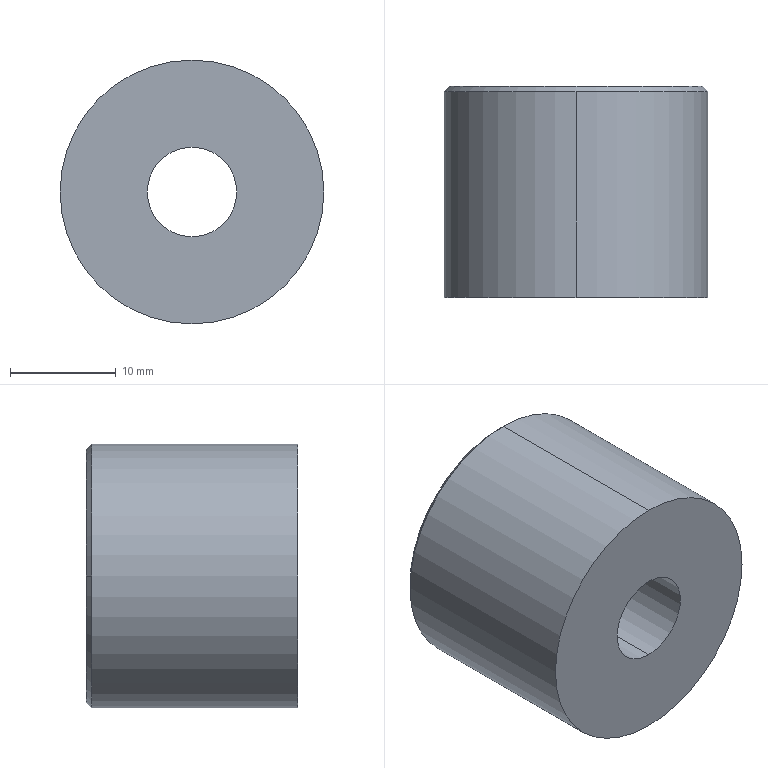Part | STEP file | VD-J260_10_1_1A_1-20_VD-SYL0380 | 1 solid | 8 faces | box 25 x 20 x 25 mm | volume 8673 mm3 | cylinder 4 | plane 2 | cone 2 | commonest cylinder face diameters 8.5 x2 25 x2
STEP:
#1=CARTESIAN_POINT('',(0.,0.,4.25));
#2=VERTEX_POINT('',#1);
#3=CARTESIAN_POINT('',(0.,0.,-4.25));
#4=VERTEX_POINT('',#3);
#5=CARTESIAN_POINT('',(0.,0.,0.));
#6=DIRECTION('',(0.,1.,0.));
#7=DIRECTION('',(0.,0.,1.));
#8=AXIS2_PLACEMENT_3D('',#5,#6,#7);
#9=CIRCLE('',#8,4.25);
#10=EDGE_CURVE('',#2,#4,#9,.T.);
#11=ORIENTED_EDGE('',*,*,#10,.F.);
#12=CARTESIAN_POINT('',(0.,20.,4.25));
#13=VERTEX_POINT('',#12);
#14=CARTESIAN_POINT('',(0.,20.,4.25));
#15=DIRECTION('',(0.,-1.,0.));
#16=VECTOR('',#15,1000.);
#17=LINE('',#14,#16);
#18=EDGE_CURVE('',#13,#2,#17,.T.);
#19=ORIENTED_EDGE('',*,*,#18,.F.);
#20=CARTESIAN_POINT('',(0.,20.,-4.25));
#21=VERTEX_POINT('',#20);
#22=CARTESIAN_POINT('',(0.,20.,0.));
#23=DIRECTION('',(0.,-1.,0.));
#24=DIRECTION('',(0.,0.,-1.));
#25=AXIS2_PLACEMENT_3D('',#22,#23,#24);
#26=CIRCLE('',#25,4.25);
#27=EDGE_CURVE('',#21,#13,#26,.T.);
#28=ORIENTED_EDGE('',*,*,#27,.F.);
#29=CARTESIAN_POINT('',(0.,20.,-4.25));
#30=DIRECTION('',(0.,-1.,0.));
#31=VECTOR('',#30,1000.);
#32=LINE('',#29,#31);
#33=EDGE_CURVE('',#21,#4,#32,.T.);
#34=ORIENTED_EDGE('',*,*,#33,.T.);
#35=EDGE_LOOP('',(#11,#19,#28,#34));
#36=FACE_OUTER_BOUND('',#35,.T.);
#37=CARTESIAN_POINT('',(0.,-14.181,0.));
#38=DIRECTION('',(0.,1.,0.));
#39=DIRECTION('',(0.,0.,1.));
#40=AXIS2_PLACEMENT_3D('',#37,#38,#39);
#41=CYLINDRICAL_SURFACE('',#40,4.25);
#42=ADVANCED_FACE('',(#36),#41,.F.);
#43=ORIENTED_EDGE('',*,*,#33,.F.);
#44=CARTESIAN_POINT('',(0.,20.,0.));
#45=DIRECTION('',(0.,-1.,0.));
#46=DIRECTION('',(0.,0.,1.));
#47=AXIS2_PLACEMENT_3D('',#44,#45,#46);
#48=CIRCLE('',#47,4.25);
#49=EDGE_CURVE('',#13,#21,#48,.T.);
#50=ORIENTED_EDGE('',*,*,#49,.F.);
#51=ORIENTED_EDGE('',*,*,#18,.T.);
#52=CARTESIAN_POINT('',(0.,0.,0.));
#53=DIRECTION('',(0.,1.,0.));
#54=DIRECTION('',(0.,0.,-1.));
#55=AXIS2_PLACEMENT_3D('',#52,#53,#54);
#56=CIRCLE('',#55,4.25);
#57=EDGE_CURVE('',#4,#2,#56,.T.);
#58=ORIENTED_EDGE('',*,*,#57,.F.);
#59=EDGE_LOOP('',(#43,#50,#51,#58));
#60=FACE_OUTER_BOUND('',#59,.T.);
#61=CARTESIAN_POINT('',(0.,-14.181,0.));
#62=DIRECTION('',(0.,1.,0.));
#63=DIRECTION('',(0.,0.,1.));
#64=AXIS2_PLACEMENT_3D('',#61,#62,#63);
#65=CYLINDRICAL_SURFACE('',#64,4.25);
#66=ADVANCED_FACE('',(#60),#65,.F.);
#67=ORIENTED_EDGE('',*,*,#10,.T.);
#68=ORIENTED_EDGE('',*,*,#57,.T.);
#69=EDGE_LOOP('',(#67,#68));
#70=FACE_BOUND('',#69,.T.);
#71=CARTESIAN_POINT('',(0.,0.,12.5));
#72=VERTEX_POINT('',#71);
#73=CARTESIAN_POINT('',(0.,0.,-12.5));
#74=VERTEX_POINT('',#73);
#75=CARTESIAN_POINT('',(0.,0.,0.));
#76=DIRECTION('',(0.,-1.,0.));
#77=DIRECTION('',(0.,0.,1.));
#78=AXIS2_PLACEMENT_3D('',#75,#76,#77);
#79=CIRCLE('',#78,12.5);
#80=EDGE_CURVE('',#72,#74,#79,.T.);
#81=ORIENTED_EDGE('',*,*,#80,.T.);
#82=CARTESIAN_POINT('',(0.,0.,0.));
#83=DIRECTION('',(0.,-1.,0.));
#84=DIRECTION('',(0.,0.,-1.));
#85=AXIS2_PLACEMENT_3D('',#82,#83,#84);
#86=CIRCLE('',#85,12.5);
#87=EDGE_CURVE('',#74,#72,#86,.T.);
#88=ORIENTED_EDGE('',*,*,#87,.T.);
#89=EDGE_LOOP('',(#81,#88));
#90=FACE_OUTER_BOUND('',#89,.T.);
#91=CARTESIAN_POINT('',(0.,0.,0.));
#92=DIRECTION('',(0.,1.,0.));
#93=DIRECTION('',(1.,0.,0.));
#94=AXIS2_PLACEMENT_3D('',#91,#92,#93);
#95=PLANE('',#94);
#96=ADVANCED_FACE('',(#70,#90),#95,.F.);
#97=CARTESIAN_POINT('',(0.,19.5,-12.5));
#98=VERTEX_POINT('',#97);
#99=CARTESIAN_POINT('',(0.,19.5,-12.5));
#100=DIRECTION('',(0.,-1.,-0.000000006));
#101=VECTOR('',#100,1000.);
#102=LINE('',#99,#101);
#103=EDGE_CURVE('',#98,#74,#102,.T.);
#104=ORIENTED_EDGE('',*,*,#103,.F.);
#105=CARTESIAN_POINT('',(12.5,19.5,0.));
#106=VERTEX_POINT('',#105);
#107=CARTESIAN_POINT('',(0.,19.5,0.));
#108=DIRECTION('',(0.,1.,0.));
#109=DIRECTION('',(1.,0.,0.));
#110=AXIS2_PLACEMENT_3D('',#107,#108,#109);
#111=CIRCLE('',#110,12.5);
#112=EDGE_CURVE('',#106,#98,#111,.T.);
#113=ORIENTED_EDGE('',*,*,#112,.F.);
#114=CARTESIAN_POINT('',(0.,19.5,12.5));
#115=VERTEX_POINT('',#114);
#116=CARTESIAN_POINT('',(0.,19.5,0.));
#117=DIRECTION('',(0.,1.,0.));
#118=DIRECTION('',(0.,0.,1.));
#119=AXIS2_PLACEMENT_3D('',#116,#117,#118);
#120=CIRCLE('',#119,12.5);
#121=EDGE_CURVE('',#115,#106,#120,.T.);
#122=ORIENTED_EDGE('',*,*,#121,.F.);
#123=CARTESIAN_POINT('',(0.,19.5,12.5));
#124=DIRECTION('',(0.,-1.,0.000000006));
#125=VECTOR('',#124,1000.);
#126=LINE('',#123,#125);
#127=EDGE_CURVE('',#115,#72,#126,.T.);
#128=ORIENTED_EDGE('',*,*,#127,.T.);
#129=ORIENTED_EDGE('',*,*,#87,.F.);
#130=EDGE_LOOP('',(#104,#113,#122,#128,#129));
#131=FACE_OUTER_BOUND('',#130,.T.);
#132=CARTESIAN_POINT('',(0.,0.,0.));
#133=DIRECTION('',(0.,1.,0.));
#134=DIRECTION('',(0.,0.,1.));
#135=AXIS2_PLACEMENT_3D('',#132,#133,#134);
#136=CYLINDRICAL_SURFACE('',#135,12.5);
#137=ADVANCED_FACE('',(#131),#136,.T.);
#138=ORIENTED_EDGE('',*,*,#80,.F.);
#139=ORIENTED_EDGE('',*,*,#127,.F.);
#140=CARTESIAN_POINT('',(-12.5,19.5,0.));
#141=VERTEX_POINT('',#140);
#142=CARTESIAN_POINT('',(0.,19.5,0.));
#143=DIRECTION('',(0.,1.,0.));
#144=DIRECTION('',(-1.,0.,0.));
#145=AXIS2_PLACEMENT_3D('',#142,#143,#144);
#146=CIRCLE('',#145,12.5);
#147=EDGE_CURVE('',#141,#115,#146,.T.);
#148=ORIENTED_EDGE('',*,*,#147,.F.);
#149=CARTESIAN_POINT('',(0.,19.5,0.));
#150=DIRECTION('',(0.,1.,0.));
#151=DIRECTION('',(0.,0.,-1.));
#152=AXIS2_PLACEMENT_3D('',#149,#150,#151);
#153=CIRCLE('',#152,12.5);
#154=EDGE_CURVE('',#98,#141,#153,.T.);
#155=ORIENTED_EDGE('',*,*,#154,.F.);
#156=ORIENTED_EDGE('',*,*,#103,.T.);
#157=EDGE_LOOP('',(#138,#139,#148,#155,#156));
#158=FACE_OUTER_BOUND('',#157,.T.);
#159=CARTESIAN_POINT('',(0.,0.,0.));
#160=DIRECTION('',(0.,1.,0.));
#161=DIRECTION('',(0.,0.,1.));
#162=AXIS2_PLACEMENT_3D('',#159,#160,#161);
#163=CYLINDRICAL_SURFACE('',#162,12.5);
#164=ADVANCED_FACE('',(#158),#163,.T.);
#165=CARTESIAN_POINT('',(12.,20.,0.));
#166=VERTEX_POINT('',#165);
#167=CARTESIAN_POINT('',(-12.,20.,0.));
#168=VERTEX_POINT('',#167);
#169=CARTESIAN_POINT('',(0.,20.,0.));
#170=DIRECTION('',(0.,1.,0.));
#171=DIRECTION('',(1.,0.,0.));
#172=AXIS2_PLACEMENT_3D('',#169,#170,#171);
#173=CIRCLE('',#172,12.);
#174=EDGE_CURVE('',#166,#168,#173,.T.);
#175=ORIENTED_EDGE('',*,*,#174,.F.);
#176=CARTESIAN_POINT('',(12.5,19.5,0.));
#177=DIRECTION('',(-0.7071,0.7071,0.));
#178=VECTOR('',#177,1000.);
#179=LINE('',#176,#178);
#180=EDGE_CURVE('',#106,#166,#179,.T.);
#181=ORIENTED_EDGE('',*,*,#180,.F.);
#182=ORIENTED_EDGE('',*,*,#112,.T.);
#183=ORIENTED_EDGE('',*,*,#154,.T.);
#184=CARTESIAN_POINT('',(-12.5,19.5,0.));
#185=DIRECTION('',(0.7071,0.7071,0.));
#186=VECTOR('',#185,1000.);
#187=LINE('',#184,#186);
#188=EDGE_CURVE('',#141,#168,#187,.T.);
#189=ORIENTED_EDGE('',*,*,#188,.T.);
#190=EDGE_LOOP('',(#175,#181,#182,#183,#189));
#191=FACE_OUTER_BOUND('',#190,.T.);
#192=CARTESIAN_POINT('',(0.,19.75,0.));
#193=DIRECTION('',(0.,-1.,0.));
#194=DIRECTION('',(1.,0.,0.));
#195=AXIS2_PLACEMENT_3D('',#192,#193,#194);
#196=CONICAL_SURFACE('',#195,12.25,0.7854);
#197=ADVANCED_FACE('',(#191),#196,.T.);
#198=ORIENTED_EDGE('',*,*,#188,.F.);
#199=ORIENTED_EDGE('',*,*,#147,.T.);
#200=ORIENTED_EDGE('',*,*,#121,.T.);
#201=ORIENTED_EDGE('',*,*,#180,.T.);
#202=CARTESIAN_POINT('',(0.,20.,0.));
#203=DIRECTION('',(0.,1.,0.));
#204=DIRECTION('',(-1.,0.,0.));
#205=AXIS2_PLACEMENT_3D('',#202,#203,#204);
#206=CIRCLE('',#205,12.);
#207=EDGE_CURVE('',#168,#166,#206,.T.);
#208=ORIENTED_EDGE('',*,*,#207,.F.);
#209=EDGE_LOOP('',(#198,#199,#200,#201,#208));
#210=FACE_OUTER_BOUND('',#209,.T.);
#211=CARTESIAN_POINT('',(0.,19.75,0.));
#212=DIRECTION('',(0.,-1.,0.));
#213=DIRECTION('',(1.,0.,0.));
#214=AXIS2_PLACEMENT_3D('',#211,#212,#213);
#215=CONICAL_SURFACE('',#214,12.25,0.7854);
#216=ADVANCED_FACE('',(#210),#215,.T.);
#217=ORIENTED_EDGE('',*,*,#27,.T.);
#218=ORIENTED_EDGE('',*,*,#49,.T.);
#219=EDGE_LOOP('',(#217,#218));
#220=FACE_BOUND('',#219,.T.);
#221=ORIENTED_EDGE('',*,*,#174,.T.);
#222=ORIENTED_EDGE('',*,*,#207,.T.);
#223=EDGE_LOOP('',(#221,#222));
#224=FACE_OUTER_BOUND('',#223,.T.);
#225=CARTESIAN_POINT('',(0.,20.,0.));
#226=DIRECTION('',(0.,1.,0.));
#227=DIRECTION('',(1.,0.,0.));
#228=AXIS2_PLACEMENT_3D('',#225,#226,#227);
#229=PLANE('',#228);
#230=ADVANCED_FACE('',(#220,#224),#229,.T.);
#231=CLOSED_SHELL('',(#42,#66,#96,#137,#164,#197,#216,#230));
#232=MANIFOLD_SOLID_BREP('',#231);
#233=CARTESIAN_POINT('',(0.,0.,0.));
#234=DIRECTION('',(0.,0.,1.));
#235=DIRECTION('',(1.,0.,0.));
#236=AXIS2_PLACEMENT_3D('',#233,#234,#235);
#237=(LENGTH_UNIT()NAMED_UNIT(*)SI_UNIT(.MILLI.,.METRE.));
#238=UNCERTAINTY_MEASURE_WITH_UNIT(LENGTH_MEASURE(0.00001),#237,'','');
#239=(NAMED_UNIT(*)PLANE_ANGLE_UNIT()SI_UNIT($,.RADIAN.));
#240=(NAMED_UNIT(*)SI_UNIT($,.STERADIAN.)SOLID_ANGLE_UNIT());
#241=(GEOMETRIC_REPRESENTATION_CONTEXT(3)GLOBAL_UNCERTAINTY_ASSIGNED_CONTEXT((#238))GLOBAL_UNIT_ASSIGNED_CONTEXT((#237,#239,#240))REPRESENTATION_CONTEXT('',''));
#242=ADVANCED_BREP_SHAPE_REPRESENTATION('',(#232,#236),#241);